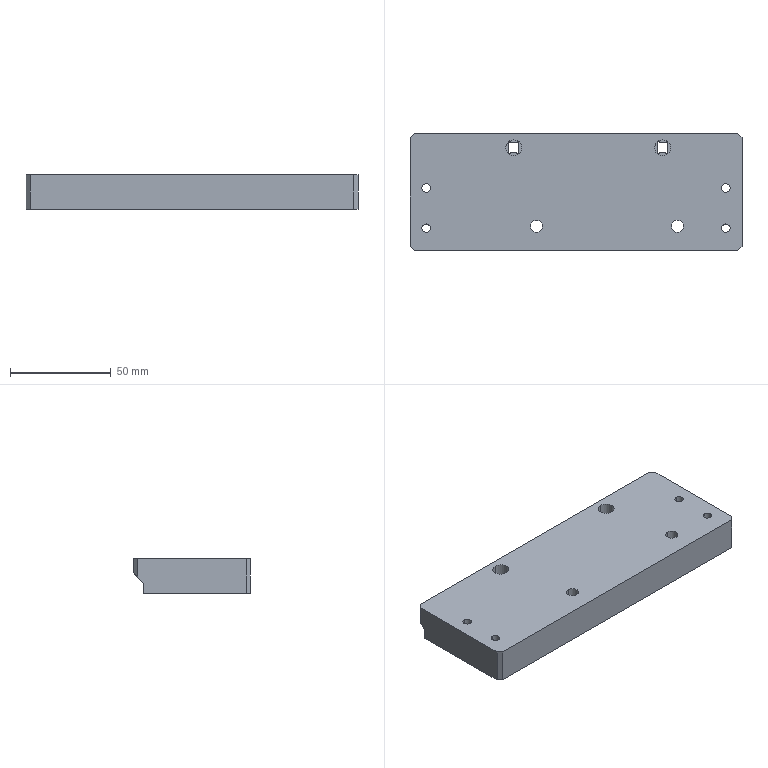NC program | NX | posted with a generic post | part box 165 x 58 x 17 mm
Lines 1652 to 3544 of 3780, first 1521 of 1881 lines:
(ZLEVEL_PROFILE_COPY_1_COPY , TOOL : D2)
N3266 T16 M6
N3268 G54
N3270 G17 G0 G90 X-1.917 Y-9.135 S9500 M3
N3272 G43 Z30. H16
N3274 Z-0.2
N3276 G94 G1 X-2.09 Y-8.835 F1000.
N3278 G3 X-2.264 Y-8.735 R0.2
N3280 G1 X-4.27
N3282 Y-10.741
N3284 G3 X-4.17 Y-10.915 R0.2
N3286 G1 X-3.87 Y-11.088
N3288 G0 X-1.917 Y-9.135 Z-0.4
N3290 G1 X-2.09 Y-8.835
N3292 G3 X-2.264 Y-8.735 R0.2
N3294 G1 X-4.27
N3296 Y-10.741
N3298 G3 X-4.17 Y-10.915 R0.2
N3300 G1 X-3.87 Y-11.088
N3302 G0 X-1.917 Y-9.135 Z-0.6
N3304 G1 X-2.09 Y-8.835
N3306 G3 X-2.264 Y-8.735 R0.2
N3308 G1 X-4.27
N3310 Y-10.741
N3312 G3 X-4.17 Y-10.915 R0.2
N3314 G1 X-3.87 Y-11.088
N3316 G0 X-1.917 Y-9.135 Z-0.8
N3318 G1 X-2.09 Y-8.835
N3320 G3 X-2.264 Y-8.735 R0.2
N3322 G1 X-4.27
N3324 Y-10.741
N3326 G3 X-4.17 Y-10.915 R0.2
N3328 G1 X-3.87 Y-11.088
N3330 G0 X-1.917 Y-9.135 Z-1.
N3332 G1 X-2.09 Y-8.835
N3334 G3 X-2.264 Y-8.735 R0.2
N3336 G1 X-4.27
N3338 Y-10.741
N3340 G3 X-4.17 Y-10.915 R0.2
N3342 G1 X-3.87 Y-11.088
N3344 G0 X-1.917 Y-9.135 Z-1.2
N3346 G1 X-2.09 Y-8.835
N3348 G3 X-2.264 Y-8.735 R0.2
N3350 G1 X-4.27
N3352 Y-10.741
N3354 G3 X-4.17 Y-10.915 R0.2
N3356 G1 X-3.87 Y-11.088
N3358 G0 X-1.917 Y-9.135 Z-1.4
N3360 G1 X-2.09 Y-8.835
N3362 G3 X-2.264 Y-8.735 R0.2
N3364 G1 X-4.27
N3366 Y-10.741
N3368 G3 X-4.17 Y-10.915 R0.2
N3370 G1 X-3.87 Y-11.088
N3372 G0 X-1.917 Y-9.135 Z-1.6
N3374 G1 X-2.09 Y-8.835
N3376 G3 X-2.264 Y-8.735 R0.2
N3378 G1 X-4.27
N3380 Y-10.741
N3382 G3 X-4.17 Y-10.915 R0.2
N3384 G1 X-3.87 Y-11.088
N3386 G0 X-1.917 Y-9.135 Z-1.8
N3388 G1 X-2.09 Y-8.835
N3390 G3 X-2.264 Y-8.735 R0.2
N3392 G1 X-4.27
N3394 Y-10.741
N3396 G3 X-4.17 Y-10.915 R0.2
N3398 G1 X-3.87 Y-11.088
N3400 G0 X-1.917 Y-9.135 Z-2.
N3402 G1 X-2.09 Y-8.835
N3404 G3 X-2.264 Y-8.735 R0.2
N3406 G1 X-4.27
N3408 Y-10.741
N3410 G3 X-4.17 Y-10.915 R0.2
N3412 G1 X-3.87 Y-11.088
N3414 G0 X-1.917 Y-9.135 Z-2.2
N3416 G1 X-2.09 Y-8.835
N3418 G3 X-2.264 Y-8.735 R0.2
N3420 G1 X-4.27
N3422 Y-10.741
N3424 G3 X-4.17 Y-10.915 R0.2
N3426 G1 X-3.87 Y-11.088
N3428 G0 X-1.917 Y-9.135 Z-2.4
N3430 G1 X-2.09 Y-8.835
N3432 G3 X-2.264 Y-8.735 R0.2
N3434 G1 X-4.27
N3436 Y-10.741
N3438 G3 X-4.17 Y-10.915 R0.2
N3440 G1 X-3.87 Y-11.088
N3442 G0 X-1.917 Y-9.135 Z-2.6
N3444 G1 X-2.09 Y-8.835
N3446 G3 X-2.264 Y-8.735 R0.2
N3448 G1 X-4.27
N3450 Y-10.741
N3452 G3 X-4.17 Y-10.915 R0.2
N3454 G1 X-3.87 Y-11.088
N3456 G0 X-1.917 Y-9.135 Z-2.8
N3458 G1 X-2.09 Y-8.835
N3460 G3 X-2.264 Y-8.735 R0.2
N3462 G1 X-4.27
N3464 Y-10.741
N3466 G3 X-4.17 Y-10.915 R0.2
N3468 G1 X-3.87 Y-11.088
N3470 G0 X-1.917 Y-9.135 Z-3.
N3472 G1 X-2.09 Y-8.835
N3474 G3 X-2.264 Y-8.735 R0.2
N3476 G1 X-4.27
N3478 Y-10.741
N3480 G3 X-4.17 Y-10.915 R0.2
N3482 G1 X-3.87 Y-11.088
N3484 G0 X-1.917 Y-9.135 Z-3.2
N3486 G1 X-2.09 Y-8.835
N3488 G3 X-2.264 Y-8.735 R0.2
N3490 G1 X-4.27
N3492 Y-10.741
N3494 G3 X-4.17 Y-10.915 R0.2
N3496 G1 X-3.87 Y-11.088
N3498 G0 X-1.917 Y-9.135 Z-3.4
N3500 G1 X-2.09 Y-8.835
N3502 G3 X-2.264 Y-8.735 R0.2
N3504 G1 X-4.27
N3506 Y-10.741
N3508 G3 X-4.17 Y-10.915 R0.2
N3510 G1 X-3.87 Y-11.088
N3512 G0 X-1.917 Y-9.135 Z-3.6
N3514 G1 X-2.09 Y-8.835
N3516 G3 X-2.264 Y-8.735 R0.2
N3518 G1 X-4.27
N3520 Y-10.741
N3522 G3 X-4.17 Y-10.915 R0.2
N3524 G1 X-3.87 Y-11.088
N3526 G0 X-1.917 Y-9.135 Z-3.8
N3528 G1 X-2.09 Y-8.835
N3530 G3 X-2.264 Y-8.735 R0.2
N3532 G1 X-4.27
N3534 Y-10.741
N3536 G3 X-4.17 Y-10.915 R0.2
N3538 G1 X-3.87 Y-11.088
N3540 G0 X-1.917 Y-9.135 Z-4.
N3542 G1 X-2.09 Y-8.835
N3544 G3 X-2.264 Y-8.735 R0.2
N3546 G1 X-4.27
N3548 Y-10.741
N3550 G3 X-4.17 Y-10.915 R0.2
N3552 G1 X-3.87 Y-11.088
N3554 G0 X-1.917 Y-9.135 Z-4.2
N3556 G1 X-2.09 Y-8.835
N3558 G3 X-2.264 Y-8.735 R0.2
N3560 G1 X-4.269
N3562 X-4.27 Y-10.741
N3564 G3 X-4.17 Y-10.915 R0.2
N3566 G1 X-3.87 Y-11.088
N3568 G0 X-1.917 Y-9.135 Z-4.4
N3570 G1 X-2.09 Y-8.835
N3572 G3 X-2.264 Y-8.735 R0.2
N3574 G1 X-4.269
N3576 X-4.27 Y-10.741
N3578 G3 X-4.17 Y-10.915 R0.2
N3580 G1 X-3.87 Y-11.088
N3582 G0 X-1.917 Y-9.135 Z-4.6
N3584 G1 X-2.09 Y-8.835
N3586 G3 X-2.264 Y-8.735 R0.2
N3588 G1 X-4.269
N3590 X-4.27 Y-10.741
N3592 G3 X-4.17 Y-10.915 R0.2
N3594 G1 X-3.87 Y-11.088
N3596 G0 X-1.917 Y-9.135 Z-4.8
N3598 G1 X-2.09 Y-8.835
N3600 G3 X-2.264 Y-8.735 R0.2
N3602 G1 X-4.269
N3604 X-4.27 Y-10.741
N3606 G3 X-4.17 Y-10.915 R0.2
N3608 G1 X-3.87 Y-11.088
N3610 G0 X-1.917 Y-9.135 Z-5.
N3612 G1 X-2.09 Y-8.835
N3614 G3 X-2.264 Y-8.735 R0.2
N3616 G1 X-4.269
N3618 X-4.27 Y-10.741
N3620 G3 X-4.17 Y-10.915 R0.2
N3622 G1 X-3.87 Y-11.088
N3624 G0 Z30.
N3626 Y-15.672
N3628 Z-0.2
N3630 G1 X-4.17 Y-15.845
N3632 G3 X-4.27 Y-16.019 R0.2
N3634 G1 Y-18.025
N3636 X-2.264
N3638 G3 X-2.09 Y-17.925 R0.2
N3640 G1 X-1.917 Y-17.625
N3642 G0 X-3.87 Y-15.672 Z-0.4
N3644 G1 X-4.17 Y-15.845
N3646 G3 X-4.27 Y-16.019 R0.2
N3648 G1 Y-18.025
N3650 X-2.264
N3652 G3 X-2.09 Y-17.925 R0.2
N3654 G1 X-1.917 Y-17.625
N3656 G0 X-3.87 Y-15.672 Z-0.6
N3658 G1 X-4.17 Y-15.845
N3660 G3 X-4.27 Y-16.019 R0.2
N3662 G1 Y-18.025
N3664 X-2.264
N3666 G3 X-2.09 Y-17.925 R0.2
N3668 G1 X-1.917 Y-17.625
N3670 G0 X-3.87 Y-15.672 Z-0.8
N3672 G1 X-4.17 Y-15.845
N3674 G3 X-4.27 Y-16.019 R0.2
N3676 G1 Y-18.025
N3678 X-2.264
N3680 G3 X-2.09 Y-17.925 R0.2
N3682 G1 X-1.917 Y-17.625
N3684 G0 X-3.87 Y-15.672 Z-1.
N3686 G1 X-4.17 Y-15.845
N3688 G3 X-4.27 Y-16.019 R0.2
N3690 G1 Y-18.025
N3692 X-2.264
N3694 G3 X-2.09 Y-17.925 R0.2
N3696 G1 X-1.917 Y-17.625
N3698 G0 X-3.87 Y-15.672 Z-1.2
N3700 G1 X-4.17 Y-15.845
N3702 G3 X-4.27 Y-16.019 R0.2
N3704 G1 Y-18.025
N3706 X-2.264
N3708 G3 X-2.09 Y-17.925 R0.2
N3710 G1 X-1.917 Y-17.625
N3712 G0 X-3.87 Y-15.672 Z-1.4
N3714 G1 X-4.17 Y-15.845
N3716 G3 X-4.27 Y-16.019 R0.2
N3718 G1 Y-18.025
N3720 X-2.264
N3722 G3 X-2.09 Y-17.925 R0.2
N3724 G1 X-1.917 Y-17.625
N3726 G0 X-3.87 Y-15.672 Z-1.6
N3728 G1 X-4.17 Y-15.845
N3730 G3 X-4.27 Y-16.019 R0.2
N3732 G1 Y-18.025
N3734 X-2.264
N3736 G3 X-2.09 Y-17.925 R0.2
N3738 G1 X-1.917 Y-17.625
N3740 G0 X-3.87 Y-15.672 Z-1.8
N3742 G1 X-4.17 Y-15.845
N3744 G3 X-4.27 Y-16.019 R0.2
N3746 G1 Y-18.025
N3748 X-2.264
N3750 G3 X-2.09 Y-17.925 R0.2
N3752 G1 X-1.917 Y-17.625
N3754 G0 X-3.87 Y-15.672 Z-2.
N3756 G1 X-4.17 Y-15.845
N3758 G3 X-4.27 Y-16.019 R0.2
N3760 G1 Y-18.025
N3762 X-2.264
N3764 G3 X-2.09 Y-17.925 R0.2
N3766 G1 X-1.917 Y-17.625
N3768 G0 X-3.87 Y-15.672 Z-2.2
N3770 G1 X-4.17 Y-15.845
N3772 G3 X-4.27 Y-16.019 R0.2
N3774 G1 Y-18.025
N3776 X-2.264
N3778 G3 X-2.09 Y-17.925 R0.2
N3780 G1 X-1.917 Y-17.625
N3782 G0 X-3.87 Y-15.672 Z-2.4
N3784 G1 X-4.17 Y-15.845
N3786 G3 X-4.27 Y-16.019 R0.2
N3788 G1 Y-18.025
N3790 X-2.264
N3792 G3 X-2.09 Y-17.925 R0.2
N3794 G1 X-1.917 Y-17.625
N3796 G0 X-3.87 Y-15.672 Z-2.6
N3798 G1 X-4.17 Y-15.845
N3800 G3 X-4.27 Y-16.019 R0.2
N3802 G1 Y-18.025
N3804 X-2.264
N3806 G3 X-2.09 Y-17.925 R0.2
N3808 G1 X-1.917 Y-17.625
N3810 G0 X-3.87 Y-15.672 Z-2.8
N3812 G1 X-4.17 Y-15.845
N3814 G3 X-4.27 Y-16.019 R0.2
N3816 G1 Y-18.025
N3818 X-2.264
N3820 G3 X-2.09 Y-17.925 R0.2
N3822 G1 X-1.917 Y-17.625
N3824 G0 X-3.87 Y-15.672 Z-3.
N3826 G1 X-4.17 Y-15.845
N3828 G3 X-4.27 Y-16.019 R0.2
N3830 G1 Y-18.025
N3832 X-2.264
N3834 G3 X-2.09 Y-17.925 R0.2
N3836 G1 X-1.917 Y-17.625
N3838 G0 X-3.87 Y-15.672 Z-3.2
N3840 G1 X-4.17 Y-15.845
N3842 G3 X-4.27 Y-16.019 R0.2
N3844 G1 Y-18.025
N3846 X-2.264
N3848 G3 X-2.09 Y-17.925 R0.2
N3850 G1 X-1.917 Y-17.625
N3852 G0 X-3.87 Y-15.672 Z-3.4
N3854 G1 X-4.17 Y-15.845
N3856 G3 X-4.27 Y-16.019 R0.2
N3858 G1 Y-18.025
N3860 X-2.264
N3862 G3 X-2.09 Y-17.925 R0.2
N3864 G1 X-1.917 Y-17.625
N3866 G0 X-3.87 Y-15.672 Z-3.6
N3868 G1 X-4.17 Y-15.845
N3870 G3 X-4.27 Y-16.019 R0.2
N3872 G1 Y-18.025
N3874 X-2.264
N3876 G3 X-2.09 Y-17.925 R0.2
N3878 G1 X-1.917 Y-17.625
N3880 G0 X-3.87 Y-15.672 Z-3.8
N3882 G1 X-4.17 Y-15.845
N3884 G3 X-4.27 Y-16.019 R0.2
N3886 G1 Y-18.025
N3888 X-2.264
N3890 G3 X-2.09 Y-17.925 R0.2
N3892 G1 X-1.917 Y-17.625
N3894 G0 X-3.87 Y-15.672 Z-4.
N3896 G1 X-4.17 Y-15.845
N3898 G3 X-4.27 Y-16.019 R0.2
N3900 G1 Y-18.025
N3902 X-2.264
N3904 G3 X-2.09 Y-17.925 R0.2
N3906 G1 X-1.917 Y-17.625
N3908 G0 X-3.87 Y-15.672 Z-4.2
N3910 G1 X-4.17 Y-15.845
N3912 G3 X-4.27 Y-16.019 R0.2
N3914 G1 Y-18.024
N3916 X-2.264 Y-18.025
N3918 G3 X-2.09 Y-17.925 R0.2
N3920 G1 X-1.917 Y-17.625
N3922 G0 X-3.87 Y-15.672 Z-4.4
N3924 G1 X-4.17 Y-15.845
N3926 G3 X-4.27 Y-16.019 R0.2
N3928 G1 Y-18.024
N3930 X-2.264 Y-18.025
N3932 G3 X-2.09 Y-17.925 R0.2
N3934 G1 X-1.917 Y-17.625
N3936 G0 X-3.87 Y-15.672 Z-4.6
N3938 G1 X-4.17 Y-15.845
N3940 G3 X-4.27 Y-16.019 R0.2
N3942 G1 Y-18.024
N3944 X-2.264 Y-18.025
N3946 G3 X-2.09 Y-17.925 R0.2
N3948 G1 X-1.917 Y-17.625
N3950 G0 X-3.87 Y-15.672 Z-4.8
N3952 G1 X-4.17 Y-15.845
N3954 G3 X-4.27 Y-16.019 R0.2
N3956 G1 Y-18.024
N3958 X-2.264 Y-18.025
N3960 G3 X-2.09 Y-17.925 R0.2
N3962 G1 X-1.917 Y-17.625
N3964 G0 X-3.87 Y-15.672 Z-5.
N3966 G1 X-4.17 Y-15.845
N3968 G3 X-4.27 Y-16.019 R0.2
N3970 G1 Y-18.024
N3972 X-2.264 Y-18.025
N3974 G3 X-2.09 Y-17.925 R0.2
N3976 G1 X-1.917 Y-17.625
N3978 G0 Z30.
N3980 X2.377
N3982 Z-0.2
N3984 G1 X2.55 Y-17.925
N3986 G3 X2.724 Y-18.025 R0.2
N3988 G1 X4.73
N3990 Y-16.019
N3992 G3 X4.63 Y-15.845 R0.2
N3994 G1 X4.33 Y-15.672
N3996 G0 X2.377 Y-17.625 Z-0.4
N3998 G1 X2.55 Y-17.925
N4000 G3 X2.724 Y-18.025 R0.2
N4002 G1 X4.73
N4004 Y-16.019
N4006 G3 X4.63 Y-15.845 R0.2
N4008 G1 X4.33 Y-15.672
N4010 G0 X2.377 Y-17.625 Z-0.6
N4012 G1 X2.55 Y-17.925
N4014 G3 X2.724 Y-18.025 R0.2
N4016 G1 X4.73
N4018 Y-16.019
N4020 G3 X4.63 Y-15.845 R0.2
N4022 G1 X4.33 Y-15.672
N4024 G0 X2.377 Y-17.625 Z-0.8
N4026 G1 X2.55 Y-17.925
N4028 G3 X2.724 Y-18.025 R0.2
N4030 G1 X4.73
N4032 Y-16.019
N4034 G3 X4.63 Y-15.845 R0.2
N4036 G1 X4.33 Y-15.672
N4038 G0 X2.377 Y-17.625 Z-1.
N4040 G1 X2.55 Y-17.925
N4042 G3 X2.724 Y-18.025 R0.2
N4044 G1 X4.73
N4046 Y-16.019
N4048 G3 X4.63 Y-15.845 R0.2
N4050 G1 X4.33 Y-15.672
N4052 G0 X2.377 Y-17.625 Z-1.2
N4054 G1 X2.55 Y-17.925
N4056 G3 X2.724 Y-18.025 R0.2
N4058 G1 X4.73
N4060 Y-16.019
N4062 G3 X4.63 Y-15.845 R0.2
N4064 G1 X4.33 Y-15.672
N4066 G0 X2.377 Y-17.625 Z-1.4
N4068 G1 X2.55 Y-17.925
N4070 G3 X2.724 Y-18.025 R0.2
N4072 G1 X4.73
N4074 Y-16.019
N4076 G3 X4.63 Y-15.845 R0.2
N4078 G1 X4.33 Y-15.672
N4080 G0 X2.377 Y-17.625 Z-1.6
N4082 G1 X2.55 Y-17.925
N4084 G3 X2.724 Y-18.025 R0.2
N4086 G1 X4.73
N4088 Y-16.019
N4090 G3 X4.63 Y-15.845 R0.2
N4092 G1 X4.33 Y-15.672
N4094 G0 X2.377 Y-17.625 Z-1.8
N4096 G1 X2.55 Y-17.925
N4098 G3 X2.724 Y-18.025 R0.2
N4100 G1 X4.73
N4102 Y-16.019
N4104 G3 X4.63 Y-15.845 R0.2
N4106 G1 X4.33 Y-15.672
N4108 G0 X2.377 Y-17.625 Z-2.
N4110 G1 X2.55 Y-17.925
N4112 G3 X2.724 Y-18.025 R0.2
N4114 G1 X4.73
N4116 Y-16.019
N4118 G3 X4.63 Y-15.845 R0.2
N4120 G1 X4.33 Y-15.672
N4122 G0 X2.377 Y-17.625 Z-2.2
N4124 G1 X2.55 Y-17.925
N4126 G3 X2.724 Y-18.025 R0.2
N4128 G1 X4.73
N4130 Y-16.019
N4132 G3 X4.63 Y-15.845 R0.2
N4134 G1 X4.33 Y-15.672
N4136 G0 X2.377 Y-17.625 Z-2.4
N4138 G1 X2.55 Y-17.925
N4140 G3 X2.724 Y-18.025 R0.2
N4142 G1 X4.73
N4144 Y-16.019
N4146 G3 X4.63 Y-15.845 R0.2
N4148 G1 X4.33 Y-15.672
N4150 G0 X2.377 Y-17.625 Z-2.6
N4152 G1 X2.55 Y-17.925
N4154 G3 X2.724 Y-18.025 R0.2
N4156 G1 X4.73
N4158 Y-16.019
N4160 G3 X4.63 Y-15.845 R0.2
N4162 G1 X4.33 Y-15.672
N4164 G0 X2.377 Y-17.625 Z-2.8
N4166 G1 X2.55 Y-17.925
N4168 G3 X2.724 Y-18.025 R0.2
N4170 G1 X4.73
N4172 Y-16.019
N4174 G3 X4.63 Y-15.845 R0.2
N4176 G1 X4.33 Y-15.672
N4178 G0 X2.377 Y-17.625 Z-3.
N4180 G1 X2.55 Y-17.925
N4182 G3 X2.724 Y-18.025 R0.2
N4184 G1 X4.73
N4186 Y-16.019
N4188 G3 X4.63 Y-15.845 R0.2
N4190 G1 X4.33 Y-15.672
N4192 G0 X2.377 Y-17.625 Z-3.2
N4194 G1 X2.55 Y-17.925
N4196 G3 X2.724 Y-18.025 R0.2
N4198 G1 X4.73
N4200 Y-16.019
N4202 G3 X4.63 Y-15.845 R0.2
N4204 G1 X4.33 Y-15.672
N4206 G0 X2.377 Y-17.625 Z-3.4
N4208 G1 X2.55 Y-17.925
N4210 G3 X2.724 Y-18.025 R0.2
N4212 G1 X4.73
N4214 Y-16.019
N4216 G3 X4.63 Y-15.845 R0.2
N4218 G1 X4.33 Y-15.672
N4220 G0 X2.377 Y-17.625 Z-3.6
N4222 G1 X2.55 Y-17.925
N4224 G3 X2.724 Y-18.025 R0.2
N4226 G1 X4.73
N4228 Y-16.019
N4230 G3 X4.63 Y-15.845 R0.2
N4232 G1 X4.33 Y-15.672
N4234 G0 X2.377 Y-17.625 Z-3.8
N4236 G1 X2.55 Y-17.925
N4238 G3 X2.724 Y-18.025 R0.2
N4240 G1 X4.73
N4242 Y-16.019
N4244 G3 X4.63 Y-15.845 R0.2
N4246 G1 X4.33 Y-15.672
N4248 G0 X2.377 Y-17.625 Z-4.
N4250 G1 X2.55 Y-17.925
N4252 G3 X2.724 Y-18.025 R0.2
N4254 G1 X4.73
N4256 Y-16.019
N4258 G3 X4.63 Y-15.845 R0.2
N4260 G1 X4.33 Y-15.672
N4262 G0 X2.377 Y-17.625 Z-4.2
N4264 G1 X2.55 Y-17.925
N4266 G3 X2.724 Y-18.025 R0.2
N4268 G1 X4.73 Y-18.024
N4270 Y-16.019
N4272 G3 X4.63 Y-15.845 R0.2
N4274 G1 X4.33 Y-15.672
N4276 G0 X2.377 Y-17.625 Z-4.4
N4278 G1 X2.55 Y-17.925
N4280 G3 X2.724 Y-18.025 R0.2
N4282 G1 X4.73 Y-18.024
N4284 Y-16.019
N4286 G3 X4.63 Y-15.845 R0.2
N4288 G1 X4.33 Y-15.672
N4290 G0 X2.377 Y-17.625 Z-4.6
N4292 G1 X2.55 Y-17.925
N4294 G3 X2.724 Y-18.025 R0.2
N4296 G1 X4.73 Y-18.024
N4298 Y-16.019
N4300 G3 X4.63 Y-15.845 R0.2
N4302 G1 X4.33 Y-15.672
N4304 G0 X2.377 Y-17.625 Z-4.8
N4306 G1 X2.55 Y-17.925
N4308 G3 X2.724 Y-18.025 R0.2
N4310 G1 X4.73 Y-18.024
N4312 Y-16.019
N4314 G3 X4.63 Y-15.845 R0.2
N4316 G1 X4.33 Y-15.672
N4318 G0 X2.377 Y-17.625 Z-5.
N4320 G1 X2.55 Y-17.925
N4322 G3 X2.724 Y-18.025 R0.2
N4324 G1 X4.73 Y-18.024
N4326 Y-16.019
N4328 G3 X4.63 Y-15.845 R0.2
N4330 G1 X4.33 Y-15.672
N4332 G0 Z30.
N4334 Y-11.088
N4336 Z-0.2
N4338 G1 X4.63 Y-10.915
N4340 G3 X4.73 Y-10.741 R0.2
N4342 G1 Y-8.735
N4344 X2.724
N4346 G3 X2.55 Y-8.835 R0.2
N4348 G1 X2.377 Y-9.135
N4350 G0 X4.33 Y-11.088 Z-0.4
N4352 G1 X4.63 Y-10.915
N4354 G3 X4.73 Y-10.741 R0.2
N4356 G1 Y-8.735
N4358 X2.724
N4360 G3 X2.55 Y-8.835 R0.2
N4362 G1 X2.377 Y-9.135
N4364 G0 X4.33 Y-11.088 Z-0.6
N4366 G1 X4.63 Y-10.915
N4368 G3 X4.73 Y-10.741 R0.2
N4370 G1 Y-8.735
N4372 X2.724
N4374 G3 X2.55 Y-8.835 R0.2
N4376 G1 X2.377 Y-9.135
N4378 G0 X4.33 Y-11.088 Z-0.8
N4380 G1 X4.63 Y-10.915
N4382 G3 X4.73 Y-10.741 R0.2
N4384 G1 Y-8.735
N4386 X2.724
N4388 G3 X2.55 Y-8.835 R0.2
N4390 G1 X2.377 Y-9.135
N4392 G0 X4.33 Y-11.088 Z-1.
N4394 G1 X4.63 Y-10.915
N4396 G3 X4.73 Y-10.741 R0.2
N4398 G1 Y-8.735
N4400 X2.724
N4402 G3 X2.55 Y-8.835 R0.2
N4404 G1 X2.377 Y-9.135
N4406 G0 X4.33 Y-11.088 Z-1.2
N4408 G1 X4.63 Y-10.915
N4410 G3 X4.73 Y-10.741 R0.2
N4412 G1 Y-8.735
N4414 X2.724
N4416 G3 X2.55 Y-8.835 R0.2
N4418 G1 X2.377 Y-9.135
N4420 G0 X4.33 Y-11.088 Z-1.4
N4422 G1 X4.63 Y-10.915
N4424 G3 X4.73 Y-10.741 R0.2
N4426 G1 Y-8.735
N4428 X2.724
N4430 G3 X2.55 Y-8.835 R0.2
N4432 G1 X2.377 Y-9.135
N4434 G0 X4.33 Y-11.088 Z-1.6
N4436 G1 X4.63 Y-10.915
N4438 G3 X4.73 Y-10.741 R0.2
N4440 G1 Y-8.735
N4442 X2.724
N4444 G3 X2.55 Y-8.835 R0.2
N4446 G1 X2.377 Y-9.135
N4448 G0 X4.33 Y-11.088 Z-1.8
N4450 G1 X4.63 Y-10.915
N4452 G3 X4.73 Y-10.741 R0.2
N4454 G1 Y-8.735
N4456 X2.724
N4458 G3 X2.55 Y-8.835 R0.2
N4460 G1 X2.377 Y-9.135
N4462 G0 X4.33 Y-11.088 Z-2.
N4464 G1 X4.63 Y-10.915
N4466 G3 X4.73 Y-10.741 R0.2
N4468 G1 Y-8.735
N4470 X2.724
N4472 G3 X2.55 Y-8.835 R0.2
N4474 G1 X2.377 Y-9.135
N4476 G0 X4.33 Y-11.088 Z-2.2
N4478 G1 X4.63 Y-10.915
N4480 G3 X4.73 Y-10.741 R0.2
N4482 G1 Y-8.735
N4484 X2.724
N4486 G3 X2.55 Y-8.835 R0.2
N4488 G1 X2.377 Y-9.135
N4490 G0 X4.33 Y-11.088 Z-2.4
N4492 G1 X4.63 Y-10.915
N4494 G3 X4.73 Y-10.741 R0.2
N4496 G1 Y-8.735
N4498 X2.724
N4500 G3 X2.55 Y-8.835 R0.2
N4502 G1 X2.377 Y-9.135
N4504 G0 X4.33 Y-11.088 Z-2.6
N4506 G1 X4.63 Y-10.915
N4508 G3 X4.73 Y-10.741 R0.2
N4510 G1 Y-8.735
N4512 X2.724
N4514 G3 X2.55 Y-8.835 R0.2
N4516 G1 X2.377 Y-9.135
N4518 G0 X4.33 Y-11.088 Z-2.8
N4520 G1 X4.63 Y-10.915
N4522 G3 X4.73 Y-10.741 R0.2
N4524 G1 Y-8.735
N4526 X2.724
N4528 G3 X2.55 Y-8.835 R0.2
N4530 G1 X2.377 Y-9.135
N4532 G0 X4.33 Y-11.088 Z-3.
N4534 G1 X4.63 Y-10.915
N4536 G3 X4.73 Y-10.741 R0.2
N4538 G1 Y-8.735
N4540 X2.724
N4542 G3 X2.55 Y-8.835 R0.2
N4544 G1 X2.377 Y-9.135
N4546 G0 X4.33 Y-11.088 Z-3.2
N4548 G1 X4.63 Y-10.915
N4550 G3 X4.73 Y-10.741 R0.2
N4552 G1 Y-8.735
N4554 X2.724
N4556 G3 X2.55 Y-8.835 R0.2
N4558 G1 X2.377 Y-9.135
N4560 G0 X4.33 Y-11.088 Z-3.4
N4562 G1 X4.63 Y-10.915
N4564 G3 X4.73 Y-10.741 R0.2
N4566 G1 Y-8.735
N4568 X2.724
N4570 G3 X2.55 Y-8.835 R0.2
N4572 G1 X2.377 Y-9.135
N4574 G0 X4.33 Y-11.088 Z-3.6
N4576 G1 X4.63 Y-10.915
N4578 G3 X4.73 Y-10.741 R0.2
N4580 G1 Y-8.735
N4582 X2.724
N4584 G3 X2.55 Y-8.835 R0.2
N4586 G1 X2.377 Y-9.135
N4588 G0 X4.33 Y-11.088 Z-3.8
N4590 G1 X4.63 Y-10.915
N4592 G3 X4.73 Y-10.741 R0.2
N4594 G1 Y-8.735
N4596 X2.724
N4598 G3 X2.55 Y-8.835 R0.2
N4600 G1 X2.377 Y-9.135
N4602 G0 X4.33 Y-11.088 Z-4.
N4604 G1 X4.63 Y-10.915
N4606 G3 X4.73 Y-10.741 R0.2
N4608 G1 Y-8.735
N4610 X2.724
N4612 G3 X2.55 Y-8.835 R0.2
N4614 G1 X2.377 Y-9.135
N4616 G0 X4.33 Y-11.088 Z-4.2
N4618 G1 X4.63 Y-10.915
N4620 G3 X4.73 Y-10.741 R0.2
N4622 G1 X4.729 Y-8.735
N4624 X2.724
N4626 G3 X2.55 Y-8.835 R0.2
N4628 G1 X2.377 Y-9.135
N4630 G0 X4.33 Y-11.088 Z-4.4
N4632 G1 X4.63 Y-10.915
N4634 G3 X4.73 Y-10.741 R0.2
N4636 G1 X4.729 Y-8.735
N4638 X2.724
N4640 G3 X2.55 Y-8.835 R0.2
N4642 G1 X2.377 Y-9.135
N4644 G0 X4.33 Y-11.088 Z-4.6
N4646 G1 X4.63 Y-10.915
N4648 G3 X4.73 Y-10.741 R0.2
N4650 G1 X4.729 Y-8.735
N4652 X2.724
N4654 G3 X2.55 Y-8.835 R0.2
N4656 G1 X2.377 Y-9.135
N4658 G0 X4.33 Y-11.088 Z-4.8
N4660 G1 X4.63 Y-10.915
N4662 G3 X4.73 Y-10.741 R0.2
N4664 G1 X4.729 Y-8.735
N4666 X2.724
N4668 G3 X2.55 Y-8.835 R0.2
N4670 G1 X2.377 Y-9.135
N4672 G0 X4.33 Y-11.088 Z-5.
N4674 G1 X4.63 Y-10.915
N4676 G3 X4.73 Y-10.741 R0.2
N4678 G1 X4.729 Y-8.735
N4680 X2.724
N4682 G3 X2.55 Y-8.835 R0.2
N4684 G1 X2.377 Y-9.135
N4686 G0 Z30.
N4688 X72.083
N4690 Z-0.2
N4692 G1 X71.91 Y-8.835
N4694 G3 X71.736 Y-8.735 R0.2
N4696 G1 X69.73
N4698 Y-10.741
N4700 G3 X69.83 Y-10.915 R0.2
N4702 G1 X70.13 Y-11.088
N4704 G0 X72.083 Y-9.135 Z-0.4
N4706 G1 X71.91 Y-8.835
N4708 G3 X71.736 Y-8.735 R0.2
N4710 G1 X69.73
N4712 Y-10.741
N4714 G3 X69.83 Y-10.915 R0.2
N4716 G1 X70.13 Y-11.088
N4718 G0 X72.083 Y-9.135 Z-0.6
N4720 G1 X71.91 Y-8.835
N4722 G3 X71.736 Y-8.735 R0.2
N4724 G1 X69.73
N4726 Y-10.741
N4728 G3 X69.83 Y-10.915 R0.2
N4730 G1 X70.13 Y-11.088
N4732 G0 X72.083 Y-9.135 Z-0.8
N4734 G1 X71.91 Y-8.835
N4736 G3 X71.736 Y-8.735 R0.2
N4738 G1 X69.73
N4740 Y-10.741
N4742 G3 X69.83 Y-10.915 R0.2
N4744 G1 X70.13 Y-11.088
N4746 G0 X72.083 Y-9.135 Z-1.
N4748 G1 X71.91 Y-8.835
N4750 G3 X71.736 Y-8.735 R0.2
N4752 G1 X69.73
N4754 Y-10.741
N4756 G3 X69.83 Y-10.915 R0.2
N4758 G1 X70.13 Y-11.088
N4760 G0 X72.083 Y-9.135 Z-1.2
N4762 G1 X71.91 Y-8.835
N4764 G3 X71.736 Y-8.735 R0.2
N4766 G1 X69.73
N4768 Y-10.741
N4770 G3 X69.83 Y-10.915 R0.2
N4772 G1 X70.13 Y-11.088
N4774 G0 X72.083 Y-9.135 Z-1.4
N4776 G1 X71.91 Y-8.835
N4778 G3 X71.736 Y-8.735 R0.2
N4780 G1 X69.73
N4782 Y-10.741
N4784 G3 X69.83 Y-10.915 R0.2
N4786 G1 X70.13 Y-11.088
N4788 G0 X72.083 Y-9.135 Z-1.6
N4790 G1 X71.91 Y-8.835
N4792 G3 X71.736 Y-8.735 R0.2
N4794 G1 X69.73
N4796 Y-10.741
N4798 G3 X69.83 Y-10.915 R0.2
N4800 G1 X70.13 Y-11.088
N4802 G0 X72.083 Y-9.135 Z-1.8
N4804 G1 X71.91 Y-8.835
N4806 G3 X71.736 Y-8.735 R0.2
N4808 G1 X69.73
N4810 Y-10.741
N4812 G3 X69.83 Y-10.915 R0.2
N4814 G1 X70.13 Y-11.088
N4816 G0 X72.083 Y-9.135 Z-2.
N4818 G1 X71.91 Y-8.835
N4820 G3 X71.736 Y-8.735 R0.2
N4822 G1 X69.73
N4824 Y-10.741
N4826 G3 X69.83 Y-10.915 R0.2
N4828 G1 X70.13 Y-11.088
N4830 G0 X72.083 Y-9.135 Z-2.2
N4832 G1 X71.91 Y-8.835
N4834 G3 X71.736 Y-8.735 R0.2
N4836 G1 X69.73
N4838 Y-10.741
N4840 G3 X69.83 Y-10.915 R0.2
N4842 G1 X70.13 Y-11.088
N4844 G0 X72.083 Y-9.135 Z-2.4
N4846 G1 X71.91 Y-8.835
N4848 G3 X71.736 Y-8.735 R0.2
N4850 G1 X69.73
N4852 Y-10.741
N4854 G3 X69.83 Y-10.915 R0.2
N4856 G1 X70.13 Y-11.088
N4858 G0 X72.083 Y-9.135 Z-2.6
N4860 G1 X71.91 Y-8.835
N4862 G3 X71.736 Y-8.735 R0.2
N4864 G1 X69.73
N4866 Y-10.741
N4868 G3 X69.83 Y-10.915 R0.2
N4870 G1 X70.13 Y-11.088
N4872 G0 X72.083 Y-9.135 Z-2.8
N4874 G1 X71.91 Y-8.835
N4876 G3 X71.736 Y-8.735 R0.2
N4878 G1 X69.73
N4880 Y-10.741
N4882 G3 X69.83 Y-10.915 R0.2
N4884 G1 X70.13 Y-11.088
N4886 G0 X72.083 Y-9.135 Z-3.
N4888 G1 X71.91 Y-8.835
N4890 G3 X71.736 Y-8.735 R0.2
N4892 G1 X69.73
N4894 Y-10.741
N4896 G3 X69.83 Y-10.915 R0.2
N4898 G1 X70.13 Y-11.088
N4900 G0 X72.083 Y-9.135 Z-3.2
N4902 G1 X71.91 Y-8.835
N4904 G3 X71.736 Y-8.735 R0.2
N4906 G1 X69.73
N4908 Y-10.741
N4910 G3 X69.83 Y-10.915 R0.2
N4912 G1 X70.13 Y-11.088
N4914 G0 X72.083 Y-9.135 Z-3.4
N4916 G1 X71.91 Y-8.835
N4918 G3 X71.736 Y-8.735 R0.2
N4920 G1 X69.73
N4922 Y-10.741
N4924 G3 X69.83 Y-10.915 R0.2
N4926 G1 X70.13 Y-11.088
N4928 G0 X72.083 Y-9.135 Z-3.6
N4930 G1 X71.91 Y-8.835
N4932 G3 X71.736 Y-8.735 R0.2
N4934 G1 X69.73
N4936 Y-10.741
N4938 G3 X69.83 Y-10.915 R0.2
N4940 G1 X70.13 Y-11.088
N4942 G0 X72.083 Y-9.135 Z-3.8
N4944 G1 X71.91 Y-8.835
N4946 G3 X71.736 Y-8.735 R0.2
N4948 G1 X69.73
N4950 Y-10.741
N4952 G3 X69.83 Y-10.915 R0.2
N4954 G1 X70.13 Y-11.088
N4956 G0 X72.083 Y-9.135 Z-4.
N4958 G1 X71.91 Y-8.835
N4960 G3 X71.736 Y-8.735 R0.2
N4962 G1 X69.73
N4964 Y-10.741
N4966 G3 X69.83 Y-10.915 R0.2
N4968 G1 X70.13 Y-11.088
N4970 G0 X72.083 Y-9.135 Z-4.2
N4972 G1 X71.91 Y-8.835
N4974 G3 X71.736 Y-8.735 R0.2
N4976 G1 X69.731
N4978 X69.73 Y-10.741
N4980 G3 X69.83 Y-10.915 R0.2
N4982 G1 X70.13 Y-11.088
N4984 G0 X72.083 Y-9.135 Z-4.4
N4986 G1 X71.91 Y-8.835
N4988 G3 X71.736 Y-8.735 R0.2
N4990 G1 X69.731
N4992 X69.73 Y-10.741
N4994 G3 X69.83 Y-10.915 R0.2
N4996 G1 X70.13 Y-11.088
N4998 G0 X72.083 Y-9.135 Z-4.6
N5000 G1 X71.91 Y-8.835
N5002 G3 X71.736 Y-8.735 R0.2
N5004 G1 X69.731
N5006 X69.73 Y-10.741
N5008 G3 X69.83 Y-10.915 R0.2
N5010 G1 X70.13 Y-11.088
N5012 G0 X72.083 Y-9.135 Z-4.8
N5014 G1 X71.91 Y-8.835
N5016 G3 X71.736 Y-8.735 R0.2
N5018 G1 X69.731
N5020 X69.73 Y-10.741
N5022 G3 X69.83 Y-10.915 R0.2
N5024 G1 X70.13 Y-11.088
N5026 G0 X72.083 Y-9.135 Z-5.
N5028 G1 X71.91 Y-8.835
N5030 G3 X71.736 Y-8.735 R0.2
N5032 G1 X69.731
N5034 X69.73 Y-10.741
N5036 G3 X69.83 Y-10.915 R0.2
N5038 G1 X70.13 Y-11.088
N5040 G0 Z30.
N5042 Y-15.672
N5044 Z-0.2
N5046 G1 X69.83 Y-15.845
N5048 G3 X69.73 Y-16.019 R0.2
N5050 G1 Y-18.025
N5052 X71.736
N5054 G3 X71.91 Y-17.925 R0.2
N5056 G1 X72.083 Y-17.625
N5058 G0 X70.13 Y-15.672 Z-0.4
N5060 G1 X69.83 Y-15.845
N5062 G3 X69.73 Y-16.018 R0.2
N5064 G1 Y-18.025
N5066 X71.737
N5068 G3 X71.91 Y-17.925 R0.2
N5070 G1 X72.083 Y-17.625
N5072 G0 X70.13 Y-15.672 Z-0.6
N5074 G1 X69.83 Y-15.845
N5076 G3 X69.73 Y-16.018 R0.2
N5078 G1 Y-18.025
N5080 X71.737
N5082 G3 X71.91 Y-17.925 R0.2
N5084 G1 X72.083 Y-17.625
N5086 G0 X70.13 Y-15.672 Z-0.8
N5088 G1 X69.83 Y-15.845
N5090 G3 X69.73 Y-16.018 R0.2
N5092 G1 Y-18.025
N5094 X71.737
N5096 G3 X71.91 Y-17.925 R0.2
N5098 G1 X72.083 Y-17.625
N5100 G0 X70.13 Y-15.672 Z-1.
N5102 G1 X69.83 Y-15.845
N5104 G3 X69.73 Y-16.018 R0.2
N5106 G1 Y-18.025
N5108 X71.737
N5110 G3 X71.91 Y-17.925 R0.2
N5112 G1 X72.083 Y-17.625
N5114 G0 X70.13 Y-15.672 Z-1.2
N5116 G1 X69.83 Y-15.845
N5118 G3 X69.73 Y-16.018 R0.2
N5120 G1 Y-18.025
N5122 X71.737
N5124 G3 X71.91 Y-17.925 R0.2
N5126 G1 X72.083 Y-17.625
N5128 G0 X70.13 Y-15.672 Z-1.4
N5130 G1 X69.83 Y-15.845
N5132 G3 X69.73 Y-16.018 R0.2
N5134 G1 Y-18.025
N5136 X71.737
N5138 G3 X71.91 Y-17.925 R0.2
N5140 G1 X72.083 Y-17.625
N5142 G0 X70.13 Y-15.672 Z-1.6
N5144 G1 X69.83 Y-15.845
N5146 G3 X69.73 Y-16.018 R0.2
N5148 G1 Y-18.025
N5150 X71.737
N5152 G3 X71.91 Y-17.925 R0.2
N5154 G1 X72.083 Y-17.625
N5156 G0 X70.13 Y-15.672 Z-1.8
N5158 G1 X69.83 Y-15.845
N5160 G3 X69.73 Y-16.018 R0.2
N5162 G1 Y-18.025
N5164 X71.737
N5166 G3 X71.91 Y-17.925 R0.2
N5168 G1 X72.083 Y-17.625
N5170 G0 X70.13 Y-15.672 Z-2.
N5172 G1 X69.83 Y-15.845
N5174 G3 X69.73 Y-16.018 R0.2
N5176 G1 Y-18.025
N5178 X71.737
N5180 G3 X71.91 Y-17.925 R0.2
N5182 G1 X72.083 Y-17.625
N5184 G0 X70.13 Y-15.672 Z-2.2
N5186 G1 X69.83 Y-15.845
N5188 G3 X69.73 Y-16.018 R0.2
N5190 G1 Y-18.025
N5192 X71.737
N5194 G3 X71.91 Y-17.925 R0.2
N5196 G1 X72.083 Y-17.625
N5198 G0 X70.13 Y-15.672 Z-2.4
N5200 G1 X69.83 Y-15.845
N5202 G3 X69.73 Y-16.018 R0.2
N5204 G1 Y-18.025
N5206 X71.737
N5208 G3 X71.91 Y-17.925 R0.2
N5210 G1 X72.083 Y-17.625
N5212 G0 X70.13 Y-15.672 Z-2.6
N5214 G1 X69.83 Y-15.845
N5216 G3 X69.73 Y-16.018 R0.2
N5218 G1 Y-18.025
N5220 X71.737
N5222 G3 X71.91 Y-17.925 R0.2
N5224 G1 X72.083 Y-17.625
N5226 G0 X70.13 Y-15.672 Z-2.8
N5228 G1 X69.83 Y-15.845
N5230 G3 X69.73 Y-16.018 R0.2
N5232 G1 Y-18.025
N5234 X71.737
N5236 G3 X71.91 Y-17.925 R0.2
N5238 G1 X72.083 Y-17.625
N5240 G0 X70.13 Y-15.672 Z-3.
N5242 G1 X69.83 Y-15.845
N5244 G3 X69.73 Y-16.018 R0.2
N5246 G1 Y-18.025
N5248 X71.737
N5250 G3 X71.91 Y-17.925 R0.2
N5252 G1 X72.083 Y-17.625
N5254 G0 X70.13 Y-15.671 Z-3.2
N5256 G1 X69.83 Y-15.845
N5258 G3 X69.73 Y-16.018 R0.2
N5260 G1 Y-18.025
N5262 X71.737
N5264 G3 X71.91 Y-17.925 R0.2
N5266 G1 X72.084 Y-17.625
N5268 G0 X70.13 Y-15.671 Z-3.4
N5270 G1 X69.83 Y-15.845
N5272 G3 X69.73 Y-16.018 R0.2
N5274 G1 Y-18.025
N5276 X71.737
N5278 G3 X71.91 Y-17.925 R0.2
N5280 G1 X72.084 Y-17.625
N5282 G0 X70.13 Y-15.671 Z-3.6
N5284 G1 X69.83 Y-15.845
N5286 G3 X69.73 Y-16.018 R0.2
N5288 G1 Y-18.025
N5290 X71.737
N5292 G3 X71.91 Y-17.925 R0.2
N5294 G1 X72.084 Y-17.625
N5296 G0 X70.13 Y-15.671 Z-3.8
N5298 G1 X69.83 Y-15.845
N5300 G3 X69.73 Y-16.018 R0.2
N5302 G1 Y-18.025
N5304 X71.737
N5306 G3 X71.91 Y-17.925 R0.2
N5308 G1 X72.084 Y-17.625
N5310 G0 X70.13 Y-15.671 Z-4.
N5312 G1 X69.83 Y-15.845
N5314 G3 X69.73 Y-16.018 R0.2
N5316 G1 Y-18.025
N5318 X71.737
N5320 G3 X71.91 Y-17.925 R0.2
N5322 G1 X72.084 Y-17.625
N5324 G0 X70.13 Y-15.671 Z-4.2
N5326 G1 X69.83 Y-15.844
N5328 G3 X69.73 Y-16.018 R0.2
N5330 G1 Y-18.024
N5332 X71.737 Y-18.025
N5334 G3 X71.911 Y-17.925 R0.2
N5336 G1 X72.084 Y-17.625
N5338 G0 X70.13 Y-15.671 Z-4.4
N5340 G1 X69.83 Y-15.844
N5342 G3 X69.73 Y-16.018 R0.2
N5344 G1 Y-18.024
N5346 X71.737 Y-18.025
N5348 G3 X71.911 Y-17.925 R0.2
N5350 G1 X72.084 Y-17.625
N5352 G0 X70.13 Y-15.671 Z-4.6
N5354 G1 X69.83 Y-15.844
N5356 G3 X69.73 Y-16.018 R0.2
N5358 G1 Y-18.024
N5360 X71.737 Y-18.025
N5362 G3 X71.911 Y-17.925 R0.2
N5364 G1 X72.084 Y-17.625
N5366 G0 X70.13 Y-15.671 Z-4.8
N5368 G1 X69.83 Y-15.844
N5370 G3 X69.73 Y-16.018 R0.2
N5372 G1 Y-18.024
N5374 X71.737 Y-18.025
N5376 G3 X71.911 Y-17.925 R0.2
N5378 G1 X72.084 Y-17.625
N5380 G0 X70.13 Y-15.671 Z-5.
N5382 G1 X69.83 Y-15.844
N5384 G3 X69.73 Y-16.018 R0.2
N5386 G1 Y-18.024
N5388 X71.738 Y-18.025
N5390 G3 X71.911 Y-17.925 R0.2
N5392 G1 X72.084 Y-17.625
N5394 G0 Z30.
N5396 X76.377
N5398 Z-0.2
N5400 G1 X76.55 Y-17.925
N5402 G3 X76.724 Y-18.025 R0.2
N5404 G1 X78.73
N5406 Y-16.019
N5408 G3 X78.63 Y-15.845 R0.2
N5410 G1 X78.33 Y-15.672
N5412 G0 X76.377 Y-17.625 Z-0.4
N5414 G1 X76.55 Y-17.925
N5416 G3 X76.724 Y-18.025 R0.2
N5418 G1 X78.73
N5420 Y-16.019
N5422 G3 X78.63 Y-15.845 R0.2
N5424 G1 X78.33 Y-15.672
N5426 G0 X76.377 Y-17.625 Z-0.6
N5428 G1 X76.55 Y-17.925
N5430 G3 X76.724 Y-18.025 R0.2
N5432 G1 X78.73
N5434 Y-16.019
N5436 G3 X78.63 Y-15.845 R0.2
N5438 G1 X78.33 Y-15.672
N5440 G0 X76.377 Y-17.625 Z-0.8
N5442 G1 X76.55 Y-17.925
N5444 G3 X76.724 Y-18.025 R0.2
N5446 G1 X78.73
N5448 Y-16.019
N5450 G3 X78.63 Y-15.845 R0.2
N5452 G1 X78.33 Y-15.672
N5454 G0 X76.377 Y-17.625 Z-1.
N5456 G1 X76.55 Y-17.925
N5458 G3 X76.724 Y-18.025 R0.2
N5460 G1 X78.73
N5462 Y-16.019
N5464 G3 X78.63 Y-15.845 R0.2
N5466 G1 X78.33 Y-15.672
N5468 G0 X76.377 Y-17.625 Z-1.2
N5470 G1 X76.55 Y-17.925
N5472 G3 X76.724 Y-18.025 R0.2
N5474 G1 X78.73
N5476 Y-16.019
N5478 G3 X78.63 Y-15.845 R0.2
N5480 G1 X78.33 Y-15.672
N5482 G0 X76.377 Y-17.625 Z-1.4
N5484 G1 X76.55 Y-17.925
N5486 G3 X76.724 Y-18.025 R0.2
N5488 G1 X78.73
N5490 Y-16.019
N5492 G3 X78.63 Y-15.845 R0.2
N5494 G1 X78.33 Y-15.672
N5496 G0 X76.377 Y-17.625 Z-1.6
N5498 G1 X76.55 Y-17.925
N5500 G3 X76.724 Y-18.025 R0.2
N5502 G1 X78.73
N5504 Y-16.019
N5506 G3 X78.63 Y-15.845 R0.2
N5508 G1 X78.33 Y-15.672
N5510 G0 X76.377 Y-17.625 Z-1.8
N5512 G1 X76.55 Y-17.925
N5514 G3 X76.724 Y-18.025 R0.2
N5516 G1 X78.73
N5518 Y-16.019
N5520 G3 X78.63 Y-15.845 R0.2
N5522 G1 X78.33 Y-15.672
N5524 G0 X76.377 Y-17.625 Z-2.
N5526 G1 X76.55 Y-17.925
N5528 G3 X76.724 Y-18.025 R0.2
N5530 G1 X78.73
N5532 Y-16.019
N5534 G3 X78.63 Y-15.845 R0.2
N5536 G1 X78.33 Y-15.672
N5538 G0 X76.377 Y-17.625 Z-2.2
N5540 G1 X76.55 Y-17.925
N5542 G3 X76.724 Y-18.025 R0.2
N5544 G1 X78.73
N5546 Y-16.019
N5548 G3 X78.63 Y-15.845 R0.2
N5550 G1 X78.33 Y-15.672
N5552 G0 X76.377 Y-17.625 Z-2.4
N5554 G1 X76.55 Y-17.925
N5556 G3 X76.724 Y-18.025 R0.2
N5558 G1 X78.73
N5560 Y-16.019
N5562 G3 X78.63 Y-15.845 R0.2
N5564 G1 X78.33 Y-15.672
N5566 G0 X76.377 Y-17.625 Z-2.6
N5568 G1 X76.55 Y-17.925
N5570 G3 X76.724 Y-18.025 R0.2
N5572 G1 X78.73
N5574 Y-16.019
N5576 G3 X78.63 Y-15.845 R0.2
N5578 G1 X78.33 Y-15.672
N5580 G0 X76.377 Y-17.625 Z-2.8
N5582 G1 X76.55 Y-17.925
N5584 G3 X76.724 Y-18.025 R0.2
N5586 G1 X78.73
N5588 Y-16.019
N5590 G3 X78.63 Y-15.845 R0.2
N5592 G1 X78.33 Y-15.672
N5594 G0 X76.377 Y-17.625 Z-3.
N5596 G1 X76.55 Y-17.925
N5598 G3 X76.724 Y-18.025 R0.2
N5600 G1 X78.73
N5602 Y-16.019
N5604 G3 X78.63 Y-15.845 R0.2
N5606 G1 X78.33 Y-15.672
N5608 G0 X76.377 Y-17.625 Z-3.2
N5610 G1 X76.55 Y-17.925
N5612 G3 X76.724 Y-18.025 R0.2
N5614 G1 X78.73
N5616 Y-16.019
N5618 G3 X78.63 Y-15.845 R0.2
N5620 G1 X78.33 Y-15.672
N5622 G0 X76.377 Y-17.625 Z-3.4
N5624 G1 X76.55 Y-17.925
N5626 G3 X76.724 Y-18.025 R0.2
N5628 G1 X78.73
N5630 Y-16.019
N5632 G3 X78.63 Y-15.845 R0.2
N5634 G1 X78.33 Y-15.672
N5636 G0 X76.377 Y-17.625 Z-3.6
N5638 G1 X76.55 Y-17.925
N5640 G3 X76.724 Y-18.025 R0.2
N5642 G1 X78.73
N5644 Y-16.019
N5646 G3 X78.63 Y-15.845 R0.2
N5648 G1 X78.33 Y-15.672
N5650 G0 X76.377 Y-17.625 Z-3.8
N5652 G1 X76.55 Y-17.925
N5654 G3 X76.724 Y-18.025 R0.2
N5656 G1 X78.73
N5658 Y-16.019
N5660 G3 X78.63 Y-15.845 R0.2
N5662 G1 X78.33 Y-15.672
N5664 G0 X76.377 Y-17.625 Z-4.
N5666 G1 X76.55 Y-17.925
N5668 G3 X76.724 Y-18.025 R0.2
N5670 G1 X78.73
N5672 Y-16.019
N5674 G3 X78.63 Y-15.845 R0.2
N5676 G1 X78.33 Y-15.672
N5678 G0 X76.377 Y-17.625 Z-4.2
N5680 G1 X76.55 Y-17.925
N5682 G3 X76.724 Y-18.025 R0.2
N5684 G1 X78.73 Y-18.024
N5686 Y-16.019
N5688 G3 X78.63 Y-15.845 R0.2
N5690 G1 X78.33 Y-15.672
N5692 G0 X76.377 Y-17.625 Z-4.4
N5694 G1 X76.55 Y-17.925
N5696 G3 X76.724 Y-18.025 R0.2
N5698 G1 X78.73 Y-18.024
N5700 Y-16.019
N5702 G3 X78.63 Y-15.845 R0.2
N5704 G1 X78.33 Y-15.672
N5706 G0 X76.377 Y-17.625 Z-4.6
N5708 G1 X76.55 Y-17.925
N5710 G3 X76.724 Y-18.025 R0.2
N5712 G1 X78.73 Y-18.024
N5714 Y-16.019
N5716 G3 X78.63 Y-15.845 R0.2
N5718 G1 X78.33 Y-15.672
N5720 G0 X76.377 Y-17.625 Z-4.8
N5722 G1 X76.55 Y-17.925
N5724 G3 X76.724 Y-18.025 R0.2
N5726 G1 X78.73 Y-18.024
N5728 Y-16.019
N5730 G3 X78.63 Y-15.845 R0.2
N5732 G1 X78.33 Y-15.672
N5734 G0 X76.377 Y-17.625 Z-5.
N5736 G1 X76.55 Y-17.925
N5738 G3 X76.724 Y-18.025 R0.2
N5740 G1 X78.73 Y-18.024
N5742 Y-16.019
N5744 G3 X78.63 Y-15.845 R0.2
N5746 G1 X78.33 Y-15.672
N5748 G0 Z30.
N5750 Y-11.088
N5752 Z-0.2
N5754 G1 X78.63 Y-10.915
N5756 G3 X78.73 Y-10.741 R0.2
N5758 G1 Y-8.735
N5760 X76.724
N5762 G3 X76.55 Y-8.835 R0.2
N5764 G1 X76.377 Y-9.135
N5766 G0 X78.33 Y-11.088 Z-0.4
N5768 G1 X78.63 Y-10.915
N5770 G3 X78.73 Y-10.741 R0.2
N5772 G1 Y-8.735
N5774 X76.724
N5776 G3 X76.55 Y-8.835 R0.2
N5778 G1 X76.377 Y-9.135
N5780 G0 X78.33 Y-11.088 Z-0.6
N5782 G1 X78.63 Y-10.915
N5784 G3 X78.73 Y-10.741 R0.2
N5786 G1 Y-8.735
N5788 X76.724
N5790 G3 X76.55 Y-8.835 R0.2
N5792 G1 X76.377 Y-9.135
N5794 G0 X78.33 Y-11.088 Z-0.8
N5796 G1 X78.63 Y-10.915
N5798 G3 X78.73 Y-10.741 R0.2
N5800 G1 Y-8.735
N5802 X76.724
N5804 G3 X76.55 Y-8.835 R0.2
N5806 G1 X76.377 Y-9.135
N5808 G0 X78.33 Y-11.088 Z-1.
N5810 G1 X78.63 Y-10.915
N5812 G3 X78.73 Y-10.741 R0.2
N5814 G1 Y-8.735
N5816 X76.724
N5818 G3 X76.55 Y-8.835 R0.2
N5820 G1 X76.377 Y-9.135
N5822 G0 X78.33 Y-11.088 Z-1.2
N5824 G1 X78.63 Y-10.915
N5826 G3 X78.73 Y-10.741 R0.2
N5828 G1 Y-8.735
N5830 X76.724
N5832 G3 X76.55 Y-8.835 R0.2
N5834 G1 X76.377 Y-9.135
N5836 G0 X78.33 Y-11.088 Z-1.4
N5838 G1 X78.63 Y-10.915
N5840 G3 X78.73 Y-10.741 R0.2
N5842 G1 Y-8.735
N5844 X76.724
N5846 G3 X76.55 Y-8.835 R0.2
N5848 G1 X76.377 Y-9.135
N5850 G0 X78.33 Y-11.088 Z-1.6
N5852 G1 X78.63 Y-10.915
N5854 G3 X78.73 Y-10.741 R0.2
N5856 G1 Y-8.735
N5858 X76.724
N5860 G3 X76.55 Y-8.835 R0.2
N5862 G1 X76.377 Y-9.135
N5864 G0 X78.33 Y-11.088 Z-1.8
N5866 G1 X78.63 Y-10.915
N5868 G3 X78.73 Y-10.741 R0.2
N5870 G1 Y-8.735
N5872 X76.724
N5874 G3 X76.55 Y-8.835 R0.2
N5876 G1 X76.377 Y-9.135
N5878 G0 X78.33 Y-11.088 Z-2.
N5880 G1 X78.63 Y-10.915
N5882 G3 X78.73 Y-10.741 R0.2
N5884 G1 Y-8.735
N5886 X76.724
N5888 G3 X76.55 Y-8.835 R0.2
N5890 G1 X76.377 Y-9.135
N5892 G0 X78.33 Y-11.088 Z-2.2
N5894 G1 X78.63 Y-10.915
N5896 G3 X78.73 Y-10.741 R0.2
N5898 G1 Y-8.735
N5900 X76.724
N5902 G3 X76.55 Y-8.835 R0.2
N5904 G1 X76.377 Y-9.135
N5906 G0 X78.33 Y-11.088 Z-2.4
N5908 G1 X78.63 Y-10.915
N5910 G3 X78.73 Y-10.741 R0.2
N5912 G1 Y-8.735
N5914 X76.724
N5916 G3 X76.55 Y-8.835 R0.2
N5918 G1 X76.377 Y-9.135
N5920 G0 X78.33 Y-11.088 Z-2.6
N5922 G1 X78.63 Y-10.915
N5924 G3 X78.73 Y-10.741 R0.2
N5926 G1 Y-8.735
N5928 X76.724
N5930 G3 X76.55 Y-8.835 R0.2
N5932 G1 X76.377 Y-9.135
N5934 G0 X78.33 Y-11.088 Z-2.8
N5936 G1 X78.63 Y-10.915
N5938 G3 X78.73 Y-10.741 R0.2
N5940 G1 Y-8.735
N5942 X76.724
N5944 G3 X76.55 Y-8.835 R0.2
N5946 G1 X76.377 Y-9.135
N5948 G0 X78.33 Y-11.088 Z-3.
N5950 G1 X78.63 Y-10.915
N5952 G3 X78.73 Y-10.741 R0.2
N5954 G1 Y-8.735
N5956 X76.724
N5958 G3 X76.55 Y-8.835 R0.2
N5960 G1 X76.377 Y-9.135
N5962 G0 X78.33 Y-11.088 Z-3.2
N5964 G1 X78.63 Y-10.915
N5966 G3 X78.73 Y-10.741 R0.2
N5968 G1 Y-8.735
N5970 X76.724
N5972 G3 X76.55 Y-8.835 R0.2
N5974 G1 X76.377 Y-9.135
N5976 G0 X78.33 Y-11.088 Z-3.4
N5978 G1 X78.63 Y-10.915
N5980 G3 X78.73 Y-10.741 R0.2
N5982 G1 Y-8.735
N5984 X76.724
N5986 G3 X76.55 Y-8.835 R0.2
N5988 G1 X76.377 Y-9.135
N5990 G0 X78.33 Y-11.088 Z-3.6
N5992 G1 X78.63 Y-10.915
N5994 G3 X78.73 Y-10.741 R0.2
N5996 G1 Y-8.735
N5998 X76.724
N6000 G3 X76.55 Y-8.835 R0.2
N6002 G1 X76.377 Y-9.135
N6004 G0 X78.33 Y-11.088 Z-3.8
N6006 G1 X78.63 Y-10.915
N6008 G3 X78.73 Y-10.741 R0.2
N6010 G1 Y-8.735
N6012 X76.724
N6014 G3 X76.55 Y-8.835 R0.2
N6016 G1 X76.377 Y-9.135
N6018 G0 X78.33 Y-11.088 Z-4.
N6020 G1 X78.63 Y-10.915
N6022 G3 X78.73 Y-10.741 R0.2
N6024 G1 Y-8.735
N6026 X76.724
N6028 G3 X76.55 Y-8.835 R0.2
N6030 G1 X76.377 Y-9.135
N6032 G0 X78.33 Y-11.088 Z-4.2
N6034 G1 X78.63 Y-10.915
N6036 G3 X78.73 Y-10.741 R0.2
N6038 G1 X78.729 Y-8.735
N6040 X76.724
N6042 G3 X76.55 Y-8.835 R0.2
N6044 G1 X76.377 Y-9.135
N6046 G0 X78.33 Y-11.088 Z-4.4
N6048 G1 X78.63 Y-10.915
N6050 G3 X78.73 Y-10.741 R0.2
N6052 G1 X78.729 Y-8.735
N6054 X76.724
N6056 G3 X76.55 Y-8.835 R0.2
N6058 G1 X76.377 Y-9.135
N6060 G0 X78.33 Y-11.088 Z-4.6
N6062 G1 X78.63 Y-10.915
N6064 G3 X78.73 Y-10.741 R0.2
N6066 G1 X78.729 Y-8.735
N6068 X76.724
N6070 G3 X76.55 Y-8.835 R0.2
N6072 G1 X76.377 Y-9.135
N6074 G0 X78.33 Y-11.088 Z-4.8
N6076 G1 X78.63 Y-10.915
N6078 G3 X78.73 Y-10.741 R0.2
N6080 G1 X78.729 Y-8.735
N6082 X76.724
N6084 G3 X76.55 Y-8.835 R0.2
N6086 G1 X76.377 Y-9.135
N6088 G0 X78.33 Y-11.088 Z-5.
N6090 G1 X78.63 Y-10.915
N6092 G3 X78.73 Y-10.741 R0.2
N6094 G1 X78.729 Y-8.735
N6096 X76.724
N6098 G3 X76.55 Y-8.835 R0.2
N6100 G1 X76.377 Y-9.135
N6102 G0 Z30.
N6104 M5
(DRILLING , TOOL : D6A45)
N6106 T01 M6
N6108 G54
N6110 G17 G0 G90 X-74.5 Y18. S9500 M3
N6112 G43 Z30. H1
N6114 G94 G81 G98 Z-1. F250. R3.
N6116 Y-2.
N6118 X-30.955 Y-21.93
N6120 X-19.62 Y17.
N6122 X50.38
N6124 X74.5 Y18.
N6126 Y-2.
N6128 X43.045 Y-21.93
N6130 G80
N6132 G0 X43.045 Y-21.93 Z30.
N6134 M5
(DRILLING_COPY_COPY , TOOL : 4.2ZT)
N6136 T04 M6
N6138 G54
N6140 G17 G0 G90 X74.5 Y-2. S2000 M3
N6142 G43 Z30. H4
N6144 G94 G83 G98 Z-19.762 F150. Q2. R3.
N6146 Y18.
N6148 X50.38 Y17.
N6150 X-19.62
N6152 X-74.5 Y18.
N6154 Y-2.
N6156 G80
N6158 G0 X-74.5 Y-2. Z30.
N6160 M5
(DRILLING_COPY_COPY_COPY , TOOL : 2.5ZT)
N6162 T02 M6
N6164 G54
N6166 G17 G0 G90 X-30.955 Y-21.93 S2000 M3
N6168 G43 Z30. H2
N6170 G94 G83 G98 Z-17.751 F150. Q2. R3.
N6172 X43.045
N6174 G80
N6176 G0 X43.045 Y-21.93 Z30.
N6178 M5
(HOLE_MILLING , TOOL : D4)
N6180 T11 M6
N6182 G54
N6184 G17 G0 G90 X-19.62 Y17. S9500 M3
N6186 G43 Z30. H11
N6188 Z0.5
N6190 G94 G3 X-19.17 Y16.55 R0.45 F1250.
N6192 X-18.72 Y17. R0.45
N6194 X-18.72 Y17. Z0.1 I-0.9 J0.
N6196 X-18.72 Y17. Z-0.3 I-0.9 J0.
N6198 X-18.72 Y17. Z-0.7 I-0.9 J0.
N6200 X-18.72 Y17. Z-1.1 I-0.9 J0.
N6202 X-18.72 Y17. Z-1.5 I-0.9 J0.
N6204 X-18.72 Y17. Z-1.9 I-0.9 J0.
N6206 X-18.72 Y17. Z-2.3 I-0.9 J0.
N6208 X-18.72 Y17. Z-2.7 I-0.9 J0.
N6210 X-18.72 Y17. Z-3.1 I-0.9 J0.
N6212 X-18.72 Y17. Z-3.5 I-0.9 J0.
N6214 X-18.72 Y17. Z-3.9 I-0.9 J0.
N6216 X-18.72 Y17. Z-4.3 I-0.9 J0.
N6218 X-18.72 Y17. Z-4.7 I-0.9 J0.
N6220 X-18.72 Y17. Z-5.1 I-0.9 J0.
N6222 X-18.72 Y17. Z-5.5 I-0.9 J0.
N6224 X-18.72 Y17. Z-5.9 I-0.9 J0.
N6226 X-18.72 Y17. Z-6.3 I-0.9 J0.
N6228 X-18.72 Y17. Z-6.7 I-0.9 J0.
N6230 X-18.72 Y17. Z-7.1 I-0.9 J0.
N6232 X-18.72 Y17. Z-7.5 I-0.9 J0.
N6234 X-18.72 Y17. Z-7.9 I-0.9 J0.
N6236 X-18.72 Y17. Z-8.3 I-0.9 J0.
N6238 X-18.72 Y17. Z-8.7 I-0.9 J0.
N6240 X-18.72 Y17. Z-9.1 I-0.9 J0.
N6242 X-18.72 Y17. Z-9.5 I-0.9 J0.
N6244 X-18.72 Y17. Z-9.9 I-0.9 J0.
N6246 X-18.72 Y17. Z-10.3 I-0.9 J0.
N6248 X-18.72 Y17. Z-10.7 I-0.9 J0.
N6250 X-18.72 Y17. Z-11.1 I-0.9 J0.
N6252 X-18.72 Y17. Z-11.5 I-0.9 J0.
N6254 X-18.72 Y17. Z-11.9 I-0.9 J0.
N6256 X-18.72 Y17. Z-12.3 I-0.9 J0.
N6258 X-18.72 Y17. Z-12.7 I-0.9 J0.
N6260 X-18.72 Y17. Z-13.1 I-0.9 J0.
N6262 X-18.72 Y17. Z-13.5 I-0.9 J0.
N6264 X-18.72 Y17. Z-13.9 I-0.9 J0.
N6266 X-18.72 Y17. Z-14.3 I-0.9 J0.
N6268 X-18.72 Y17. Z-14.7 I-0.9 J0.
N6270 X-18.72 Y17. Z-15.1 I-0.9 J0.
N6272 X-18.72 Y17. Z-15.5 I-0.9 J0.
N6274 X-18.72 Y17. Z-15.9 I-0.9 J0.
N6276 X-18.72 Y17. Z-16.3 I-0.9 J0.
N6278 X-18.72 Y17. Z-16.7 I-0.9 J0.
N6280 X-19.62 Y16.1 Z-17. R-0.9
N6282 X-18.72 Y17. R0.9
N6284 X-19.62 Y16.1 R-0.9
N6286 X-19.17 Y16.55 R0.45
N6288 X-19.62 Y17. R0.45
N6290 G0 Z30.
N6292 X50.38
N6294 Z0.5
N6296 G3 X50.83 Y16.55 R0.45